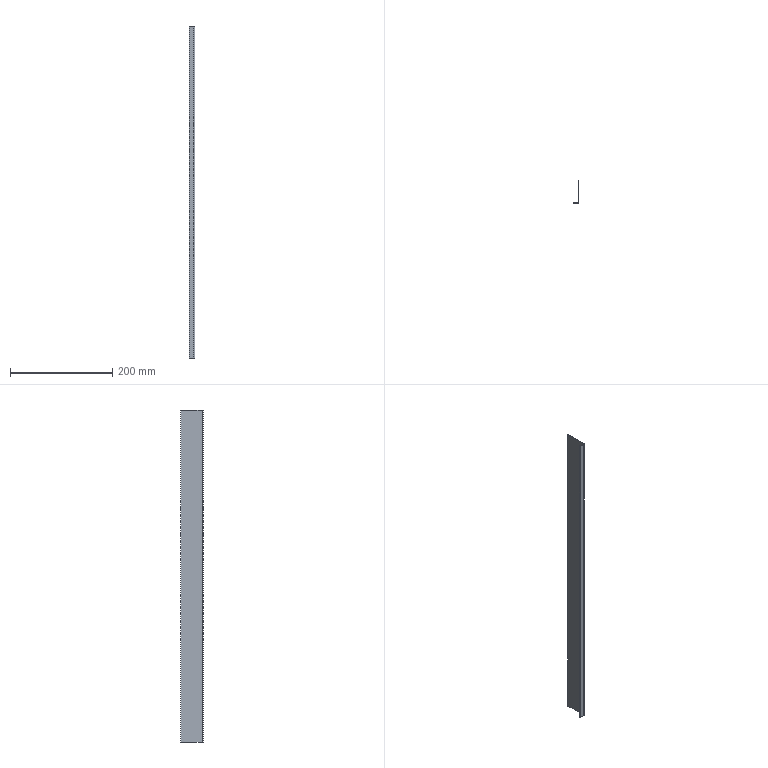Part | STEP file | 001-010-Waste drag chain mounting sheet metal | 1 solid | 14 faces | box 11.5 x 44.5 x 650 mm | volume 52405 mm3 | plane 12 | cylinder 2 | commonest cylinder face diameters 2 x1 5 x1
STEP:
#1=CARTESIAN_POINT('',(0.,0.,0.));
#2=DIRECTION('',(0.,0.,1.));
#3=DIRECTION('',(1.,0.,0.));
#4=AXIS2_PLACEMENT_3D('',#1,#2,#3);
#5=CARTESIAN_POINT('',(0.,1.,325.));
#6=VERTEX_POINT('',#5);
#7=CARTESIAN_POINT('',(1.5,1.,325.));
#8=VERTEX_POINT('',#7);
#9=CARTESIAN_POINT('',(0.,1.,325.));
#10=DIRECTION('',(1.,0.,0.));
#11=VECTOR('',#10,1.);
#12=LINE('',#9,#11);
#13=CARTESIAN_POINT('',(0.,1.,325.));
#14=DIRECTION('',(0.,0.,1.));
#15=DIRECTION('',(1.,0.,0.));
#16=AXIS2_PLACEMENT_3D('',#13,#14,#15);
#17=PLANE('',#16);
#18=CARTESIAN_POINT('',(0.,0.));
#19=DIRECTION('',(1.,0.));
#20=VECTOR('',#19,1.);
#21=LINE('',#18,#20);
#22=(GEOMETRIC_REPRESENTATION_CONTEXT(2)PARAMETRIC_REPRESENTATION_CONTEXT()REPRESENTATION_CONTEXT('',''));
#23=DEFINITIONAL_REPRESENTATION('',(#21),#22);
#24=PCURVE('',#17,#23);
#25=CARTESIAN_POINT('',(-1.,-1.5,325.));
#26=DIRECTION('',(0.,0.,1.));
#27=DIRECTION('',(1.,0.,0.));
#28=AXIS2_PLACEMENT_3D('',#25,#26,#27);
#29=PLANE('',#28);
#30=CARTESIAN_POINT('',(1.,2.5));
#31=DIRECTION('',(1.,0.));
#32=VECTOR('',#31,1.);
#33=LINE('',#30,#32);
#34=(GEOMETRIC_REPRESENTATION_CONTEXT(2)PARAMETRIC_REPRESENTATION_CONTEXT()REPRESENTATION_CONTEXT('',''));
#35=DEFINITIONAL_REPRESENTATION('',(#33),#34);
#36=PCURVE('',#29,#35);
#37=SURFACE_CURVE('',#12,(#24,#36),.PCURVE_S1.);
#38=EDGE_CURVE('',#6,#8,#37,.T.);
#39=ORIENTED_EDGE('',*,*,#38,.F.);
#40=CARTESIAN_POINT('',(-1.,0.,325.));
#41=VERTEX_POINT('',#40);
#42=CARTESIAN_POINT('',(-1.,1.,325.));
#43=DIRECTION('',(0.,0.,1.));
#44=DIRECTION('',(-1.,0.,0.));
#45=AXIS2_PLACEMENT_3D('',#42,#43,#44);
#46=CIRCLE('',#45,1.);
#47=CARTESIAN_POINT('',(-1.,0.));
#48=DIRECTION('',(-1.,0.));
#49=AXIS2_PLACEMENT_2D('',#47,#48);
#50=CIRCLE('',#49,1.);
#51=(GEOMETRIC_REPRESENTATION_CONTEXT(2)PARAMETRIC_REPRESENTATION_CONTEXT()REPRESENTATION_CONTEXT('',''));
#52=DEFINITIONAL_REPRESENTATION('',(#50),#51);
#53=PCURVE('',#17,#52);
#54=CARTESIAN_POINT('',(-1.,1.,325.));
#55=DIRECTION('',(0.,0.,-1.));
#56=DIRECTION('',(-1.,0.,0.));
#57=AXIS2_PLACEMENT_3D('',#54,#55,#56);
#58=CYLINDRICAL_SURFACE('',#57,1.);
#59=CARTESIAN_POINT('',(6.283,0.));
#60=DIRECTION('',(-1.,0.));
#61=VECTOR('',#60,1.);
#62=LINE('',#59,#61);
#63=(GEOMETRIC_REPRESENTATION_CONTEXT(2)PARAMETRIC_REPRESENTATION_CONTEXT()REPRESENTATION_CONTEXT('',''));
#64=DEFINITIONAL_REPRESENTATION('',(#62),#63);
#65=PCURVE('',#58,#64);
#66=SURFACE_CURVE('',#46,(#53,#65),.PCURVE_S1.);
#67=EDGE_CURVE('',#41,#6,#66,.T.);
#68=ORIENTED_EDGE('',*,*,#67,.F.);
#69=CARTESIAN_POINT('',(-1.,-1.5,325.));
#70=VERTEX_POINT('',#69);
#71=CARTESIAN_POINT('',(-1.,-1.5,325.));
#72=DIRECTION('',(0.,1.,0.));
#73=VECTOR('',#72,1.);
#74=LINE('',#71,#73);
#75=CARTESIAN_POINT('',(-1.,-2.5));
#76=DIRECTION('',(0.,1.));
#77=VECTOR('',#76,1.);
#78=LINE('',#75,#77);
#79=(GEOMETRIC_REPRESENTATION_CONTEXT(2)PARAMETRIC_REPRESENTATION_CONTEXT()REPRESENTATION_CONTEXT('',''));
#80=DEFINITIONAL_REPRESENTATION('',(#78),#79);
#81=PCURVE('',#17,#80);
#82=CARTESIAN_POINT('',(-1.,1.,325.));
#83=DIRECTION('',(0.,0.,-1.));
#84=DIRECTION('',(-1.,0.,0.));
#85=AXIS2_PLACEMENT_3D('',#82,#83,#84);
#86=PLANE('',#85);
#87=CARTESIAN_POINT('',(0.,-2.5));
#88=DIRECTION('',(0.,1.));
#89=VECTOR('',#88,1.);
#90=LINE('',#87,#89);
#91=(GEOMETRIC_REPRESENTATION_CONTEXT(2)PARAMETRIC_REPRESENTATION_CONTEXT()REPRESENTATION_CONTEXT('',''));
#92=DEFINITIONAL_REPRESENTATION('',(#90),#91);
#93=PCURVE('',#86,#92);
#94=SURFACE_CURVE('',#74,(#81,#93),.PCURVE_S1.);
#95=EDGE_CURVE('',#70,#41,#94,.T.);
#96=ORIENTED_EDGE('',*,*,#95,.F.);
#97=CARTESIAN_POINT('',(-1.,1.,325.));
#98=DIRECTION('',(0.,0.,1.));
#99=DIRECTION('',(1.,0.,0.));
#100=AXIS2_PLACEMENT_3D('',#97,#98,#99);
#101=CIRCLE('',#100,2.5);
#102=CARTESIAN_POINT('',(-1.,0.));
#103=DIRECTION('',(1.,0.));
#104=AXIS2_PLACEMENT_2D('',#102,#103);
#105=CIRCLE('',#104,2.5);
#106=(GEOMETRIC_REPRESENTATION_CONTEXT(2)PARAMETRIC_REPRESENTATION_CONTEXT()REPRESENTATION_CONTEXT('',''));
#107=DEFINITIONAL_REPRESENTATION('',(#105),#106);
#108=PCURVE('',#17,#107);
#109=CARTESIAN_POINT('',(-1.,1.,325.));
#110=DIRECTION('',(0.,0.,-1.));
#111=DIRECTION('',(-1.,0.,0.));
#112=AXIS2_PLACEMENT_3D('',#109,#110,#111);
#113=CYLINDRICAL_SURFACE('',#112,2.5);
#114=CARTESIAN_POINT('',(9.425,0.));
#115=DIRECTION('',(-1.,0.));
#116=VECTOR('',#115,1.);
#117=LINE('',#114,#116);
#118=(GEOMETRIC_REPRESENTATION_CONTEXT(2)PARAMETRIC_REPRESENTATION_CONTEXT()REPRESENTATION_CONTEXT('',''));
#119=DEFINITIONAL_REPRESENTATION('',(#117),#118);
#120=PCURVE('',#113,#119);
#121=SURFACE_CURVE('',#101,(#108,#120),.PCURVE_S1.);
#122=EDGE_CURVE('',#70,#8,#121,.T.);
#123=ORIENTED_EDGE('',*,*,#122,.T.);
#124=EDGE_LOOP('',(#39,#68,#96,#123));
#125=FACE_BOUND('',#124,.T.);
#126=ADVANCED_FACE('',(#125),#17,.T.);
#127=CARTESIAN_POINT('',(0.,43.,325.));
#128=VERTEX_POINT('',#127);
#129=CARTESIAN_POINT('',(0.,0.,325.));
#130=DIRECTION('',(0.,1.,0.));
#131=VECTOR('',#130,1.);
#132=LINE('',#129,#131);
#133=CARTESIAN_POINT('',(1.,1.5));
#134=DIRECTION('',(0.,1.));
#135=VECTOR('',#134,1.);
#136=LINE('',#133,#135);
#137=(GEOMETRIC_REPRESENTATION_CONTEXT(2)PARAMETRIC_REPRESENTATION_CONTEXT()REPRESENTATION_CONTEXT('',''));
#138=DEFINITIONAL_REPRESENTATION('',(#136),#137);
#139=PCURVE('',#29,#138);
#140=CARTESIAN_POINT('',(0.,0.,325.));
#141=DIRECTION('',(-1.,0.,0.));
#142=DIRECTION('',(0.,0.,1.));
#143=AXIS2_PLACEMENT_3D('',#140,#141,#142);
#144=PLANE('',#143);
#145=CARTESIAN_POINT('',(0.,0.));
#146=DIRECTION('',(0.,1.));
#147=VECTOR('',#146,1.);
#148=LINE('',#145,#147);
#149=(GEOMETRIC_REPRESENTATION_CONTEXT(2)PARAMETRIC_REPRESENTATION_CONTEXT()REPRESENTATION_CONTEXT('',''));
#150=DEFINITIONAL_REPRESENTATION('',(#148),#149);
#151=PCURVE('',#144,#150);
#152=SURFACE_CURVE('',#132,(#139,#151),.PCURVE_S1.);
#153=EDGE_CURVE('',#6,#128,#152,.T.);
#154=ORIENTED_EDGE('',*,*,#153,.F.);
#155=ORIENTED_EDGE('',*,*,#38,.T.);
#156=CARTESIAN_POINT('',(1.5,43.,325.));
#157=VERTEX_POINT('',#156);
#158=CARTESIAN_POINT('',(1.5,0.,325.));
#159=DIRECTION('',(0.,1.,0.));
#160=VECTOR('',#159,1.);
#161=LINE('',#158,#160);
#162=CARTESIAN_POINT('',(2.5,1.5));
#163=DIRECTION('',(0.,1.));
#164=VECTOR('',#163,1.);
#165=LINE('',#162,#164);
#166=(GEOMETRIC_REPRESENTATION_CONTEXT(2)PARAMETRIC_REPRESENTATION_CONTEXT()REPRESENTATION_CONTEXT('',''));
#167=DEFINITIONAL_REPRESENTATION('',(#165),#166);
#168=PCURVE('',#29,#167);
#169=CARTESIAN_POINT('',(1.5,0.,325.));
#170=DIRECTION('',(-1.,0.,0.));
#171=DIRECTION('',(0.,0.,1.));
#172=AXIS2_PLACEMENT_3D('',#169,#170,#171);
#173=PLANE('',#172);
#174=CARTESIAN_POINT('',(0.,0.));
#175=DIRECTION('',(0.,1.));
#176=VECTOR('',#175,1.);
#177=LINE('',#174,#176);
#178=(GEOMETRIC_REPRESENTATION_CONTEXT(2)PARAMETRIC_REPRESENTATION_CONTEXT()REPRESENTATION_CONTEXT('',''));
#179=DEFINITIONAL_REPRESENTATION('',(#177),#178);
#180=PCURVE('',#173,#179);
#181=SURFACE_CURVE('',#161,(#168,#180),.PCURVE_S1.);
#182=EDGE_CURVE('',#8,#157,#181,.T.);
#183=ORIENTED_EDGE('',*,*,#182,.T.);
#184=CARTESIAN_POINT('',(0.,43.,325.));
#185=DIRECTION('',(1.,0.,0.));
#186=VECTOR('',#185,1.);
#187=LINE('',#184,#186);
#188=CARTESIAN_POINT('',(1.,44.5));
#189=DIRECTION('',(1.,0.));
#190=VECTOR('',#189,1.);
#191=LINE('',#188,#190);
#192=(GEOMETRIC_REPRESENTATION_CONTEXT(2)PARAMETRIC_REPRESENTATION_CONTEXT()REPRESENTATION_CONTEXT('',''));
#193=DEFINITIONAL_REPRESENTATION('',(#191),#192);
#194=PCURVE('',#29,#193);
#195=CARTESIAN_POINT('',(0.,43.,325.));
#196=DIRECTION('',(0.,1.,0.));
#197=DIRECTION('',(0.,0.,1.));
#198=AXIS2_PLACEMENT_3D('',#195,#196,#197);
#199=PLANE('',#198);
#200=CARTESIAN_POINT('',(0.,0.));
#201=DIRECTION('',(0.,1.));
#202=VECTOR('',#201,1.);
#203=LINE('',#200,#202);
#204=(GEOMETRIC_REPRESENTATION_CONTEXT(2)PARAMETRIC_REPRESENTATION_CONTEXT()REPRESENTATION_CONTEXT('',''));
#205=DEFINITIONAL_REPRESENTATION('',(#203),#204);
#206=PCURVE('',#199,#205);
#207=SURFACE_CURVE('',#187,(#194,#206),.PCURVE_S1.);
#208=EDGE_CURVE('',#128,#157,#207,.T.);
#209=ORIENTED_EDGE('',*,*,#208,.F.);
#210=EDGE_LOOP('',(#154,#155,#183,#209));
#211=FACE_BOUND('',#210,.T.);
#212=ADVANCED_FACE('',(#211),#29,.T.);
#213=CARTESIAN_POINT('',(-1.,0.,-325.));
#214=VERTEX_POINT('',#213);
#215=CARTESIAN_POINT('',(-1.,-1.5,-325.));
#216=VERTEX_POINT('',#215);
#217=CARTESIAN_POINT('',(-1.,0.,-325.));
#218=DIRECTION('',(0.,-1.,0.));
#219=VECTOR('',#218,1.);
#220=LINE('',#217,#219);
#221=CARTESIAN_POINT('',(-1.,0.,-325.));
#222=DIRECTION('',(0.,0.,-1.));
#223=DIRECTION('',(-1.,0.,0.));
#224=AXIS2_PLACEMENT_3D('',#221,#222,#223);
#225=PLANE('',#224);
#226=CARTESIAN_POINT('',(0.,0.));
#227=DIRECTION('',(0.,-1.));
#228=VECTOR('',#227,1.);
#229=LINE('',#226,#228);
#230=(GEOMETRIC_REPRESENTATION_CONTEXT(2)PARAMETRIC_REPRESENTATION_CONTEXT()REPRESENTATION_CONTEXT('',''));
#231=DEFINITIONAL_REPRESENTATION('',(#229),#230);
#232=PCURVE('',#225,#231);
#233=CARTESIAN_POINT('',(1.5,1.,-325.));
#234=DIRECTION('',(0.,0.,-1.));
#235=DIRECTION('',(-1.,0.,0.));
#236=AXIS2_PLACEMENT_3D('',#233,#234,#235);
#237=PLANE('',#236);
#238=CARTESIAN_POINT('',(2.5,-1.));
#239=DIRECTION('',(0.,-1.));
#240=VECTOR('',#239,1.);
#241=LINE('',#238,#240);
#242=(GEOMETRIC_REPRESENTATION_CONTEXT(2)PARAMETRIC_REPRESENTATION_CONTEXT()REPRESENTATION_CONTEXT('',''));
#243=DEFINITIONAL_REPRESENTATION('',(#241),#242);
#244=PCURVE('',#237,#243);
#245=SURFACE_CURVE('',#220,(#232,#244),.PCURVE_S1.);
#246=EDGE_CURVE('',#214,#216,#245,.T.);
#247=ORIENTED_EDGE('',*,*,#246,.F.);
#248=CARTESIAN_POINT('',(0.,1.,-325.));
#249=VERTEX_POINT('',#248);
#250=CARTESIAN_POINT('',(-1.,1.,-325.));
#251=DIRECTION('',(0.,0.,1.));
#252=DIRECTION('',(-1.,0.,0.));
#253=AXIS2_PLACEMENT_3D('',#250,#251,#252);
#254=CIRCLE('',#253,1.);
#255=CARTESIAN_POINT('',(1.,1.));
#256=CARTESIAN_POINT('',(1.,-0.7321));
#257=CARTESIAN_POINT('',(-0.5,0.134));
#258=CARTESIAN_POINT('',(-2.,1.));
#259=CARTESIAN_POINT('',(-0.5,1.866));
#260=CARTESIAN_POINT('',(1.,2.732));
#261=CARTESIAN_POINT('',(1.,1.));
#262=(BOUNDED_CURVE()B_SPLINE_CURVE(2,(#255,#256,#257,#258,#259,#260,#261),.UNSPECIFIED.,.T.,.F.)B_SPLINE_CURVE_WITH_KNOTS((1,2,2,2,2,1),(-2.094,0.,2.094,4.189,6.283,8.378),.UNSPECIFIED.)CURVE()GEOMETRIC_REPRESENTATION_ITEM()RATIONAL_B_SPLINE_CURVE((1.,0.5,1.,0.5,1.,0.5,1.))REPRESENTATION_ITEM(''));
#263=(GEOMETRIC_REPRESENTATION_CONTEXT(2)PARAMETRIC_REPRESENTATION_CONTEXT()REPRESENTATION_CONTEXT('',''));
#264=DEFINITIONAL_REPRESENTATION('',(#262),#263);
#265=PCURVE('',#225,#264);
#266=CARTESIAN_POINT('',(6.283,650.));
#267=DIRECTION('',(-1.,0.));
#268=VECTOR('',#267,1.);
#269=LINE('',#266,#268);
#270=(GEOMETRIC_REPRESENTATION_CONTEXT(2)PARAMETRIC_REPRESENTATION_CONTEXT()REPRESENTATION_CONTEXT('',''));
#271=DEFINITIONAL_REPRESENTATION('',(#269),#270);
#272=PCURVE('',#58,#271);
#273=SURFACE_CURVE('',#254,(#265,#272),.PCURVE_S1.);
#274=EDGE_CURVE('',#214,#249,#273,.T.);
#275=ORIENTED_EDGE('',*,*,#274,.T.);
#276=CARTESIAN_POINT('',(1.5,1.,-325.));
#277=VERTEX_POINT('',#276);
#278=CARTESIAN_POINT('',(1.5,1.,-325.));
#279=DIRECTION('',(-1.,0.,0.));
#280=VECTOR('',#279,1.);
#281=LINE('',#278,#280);
#282=CARTESIAN_POINT('',(-2.5,1.));
#283=DIRECTION('',(1.,0.));
#284=VECTOR('',#283,1.);
#285=LINE('',#282,#284);
#286=(GEOMETRIC_REPRESENTATION_CONTEXT(2)PARAMETRIC_REPRESENTATION_CONTEXT()REPRESENTATION_CONTEXT('',''));
#287=DEFINITIONAL_REPRESENTATION('',(#285),#286);
#288=PCURVE('',#225,#287);
#289=CARTESIAN_POINT('',(-1.,1.,-325.));
#290=DIRECTION('',(0.,0.,-1.));
#291=DIRECTION('',(-1.,0.,0.));
#292=AXIS2_PLACEMENT_3D('',#289,#290,#291);
#293=PLANE('',#292);
#294=CARTESIAN_POINT('',(-2.5,0.));
#295=DIRECTION('',(1.,0.));
#296=VECTOR('',#295,1.);
#297=LINE('',#294,#296);
#298=(GEOMETRIC_REPRESENTATION_CONTEXT(2)PARAMETRIC_REPRESENTATION_CONTEXT()REPRESENTATION_CONTEXT('',''));
#299=DEFINITIONAL_REPRESENTATION('',(#297),#298);
#300=PCURVE('',#293,#299);
#301=SURFACE_CURVE('',#281,(#288,#300),.PCURVE_S1.);
#302=EDGE_CURVE('',#277,#249,#301,.T.);
#303=ORIENTED_EDGE('',*,*,#302,.F.);
#304=CARTESIAN_POINT('',(-1.,1.,-325.));
#305=DIRECTION('',(0.,0.,1.));
#306=DIRECTION('',(1.,0.,0.));
#307=AXIS2_PLACEMENT_3D('',#304,#305,#306);
#308=CIRCLE('',#307,2.5);
#309=CARTESIAN_POINT('',(-2.5,1.));
#310=CARTESIAN_POINT('',(-2.5,5.33));
#311=CARTESIAN_POINT('',(1.25,3.165));
#312=CARTESIAN_POINT('',(5.,1.));
#313=CARTESIAN_POINT('',(1.25,-1.165));
#314=CARTESIAN_POINT('',(-2.5,-3.33));
#315=CARTESIAN_POINT('',(-2.5,1.));
#316=(BOUNDED_CURVE()B_SPLINE_CURVE(2,(#309,#310,#311,#312,#313,#314,#315),.UNSPECIFIED.,.T.,.F.)B_SPLINE_CURVE_WITH_KNOTS((1,2,2,2,2,1),(-2.094,0.,2.094,4.189,6.283,8.378),.UNSPECIFIED.)CURVE()GEOMETRIC_REPRESENTATION_ITEM()RATIONAL_B_SPLINE_CURVE((1.,0.5,1.,0.5,1.,0.5,1.))REPRESENTATION_ITEM(''));
#317=(GEOMETRIC_REPRESENTATION_CONTEXT(2)PARAMETRIC_REPRESENTATION_CONTEXT()REPRESENTATION_CONTEXT('',''));
#318=DEFINITIONAL_REPRESENTATION('',(#316),#317);
#319=PCURVE('',#225,#318);
#320=CARTESIAN_POINT('',(9.425,650.));
#321=DIRECTION('',(-1.,0.));
#322=VECTOR('',#321,1.);
#323=LINE('',#320,#322);
#324=(GEOMETRIC_REPRESENTATION_CONTEXT(2)PARAMETRIC_REPRESENTATION_CONTEXT()REPRESENTATION_CONTEXT('',''));
#325=DEFINITIONAL_REPRESENTATION('',(#323),#324);
#326=PCURVE('',#113,#325);
#327=SURFACE_CURVE('',#308,(#319,#326),.PCURVE_S1.);
#328=EDGE_CURVE('',#216,#277,#327,.T.);
#329=ORIENTED_EDGE('',*,*,#328,.F.);
#330=EDGE_LOOP('',(#247,#275,#303,#329));
#331=FACE_BOUND('',#330,.T.);
#332=ADVANCED_FACE('',(#331),#225,.T.);
#333=CARTESIAN_POINT('',(-10.,0.,-325.));
#334=VERTEX_POINT('',#333);
#335=CARTESIAN_POINT('',(0.,0.,-325.));
#336=DIRECTION('',(1.,0.,0.));
#337=VECTOR('',#336,1.);
#338=LINE('',#335,#337);
#339=CARTESIAN_POINT('',(1.5,-1.));
#340=DIRECTION('',(-1.,0.));
#341=VECTOR('',#340,1.);
#342=LINE('',#339,#341);
#343=(GEOMETRIC_REPRESENTATION_CONTEXT(2)PARAMETRIC_REPRESENTATION_CONTEXT()REPRESENTATION_CONTEXT('',''));
#344=DEFINITIONAL_REPRESENTATION('',(#342),#343);
#345=PCURVE('',#237,#344);
#346=CARTESIAN_POINT('',(0.,0.,325.));
#347=DIRECTION('',(0.,1.,0.));
#348=DIRECTION('',(0.,0.,1.));
#349=AXIS2_PLACEMENT_3D('',#346,#347,#348);
#350=PLANE('',#349);
#351=CARTESIAN_POINT('',(-650.,0.));
#352=DIRECTION('',(0.,1.));
#353=VECTOR('',#352,1.);
#354=LINE('',#351,#353);
#355=(GEOMETRIC_REPRESENTATION_CONTEXT(2)PARAMETRIC_REPRESENTATION_CONTEXT()REPRESENTATION_CONTEXT('',''));
#356=DEFINITIONAL_REPRESENTATION('',(#354),#355);
#357=PCURVE('',#350,#356);
#358=SURFACE_CURVE('',#338,(#345,#357),.PCURVE_S1.);
#359=EDGE_CURVE('',#334,#214,#358,.T.);
#360=ORIENTED_EDGE('',*,*,#359,.T.);
#361=ORIENTED_EDGE('',*,*,#246,.T.);
#362=CARTESIAN_POINT('',(-10.,-1.5,-325.));
#363=VERTEX_POINT('',#362);
#364=CARTESIAN_POINT('',(0.,-1.5,-325.));
#365=DIRECTION('',(1.,0.,0.));
#366=VECTOR('',#365,1.);
#367=LINE('',#364,#366);
#368=CARTESIAN_POINT('',(1.5,-2.5));
#369=DIRECTION('',(-1.,0.));
#370=VECTOR('',#369,1.);
#371=LINE('',#368,#370);
#372=(GEOMETRIC_REPRESENTATION_CONTEXT(2)PARAMETRIC_REPRESENTATION_CONTEXT()REPRESENTATION_CONTEXT('',''));
#373=DEFINITIONAL_REPRESENTATION('',(#371),#372);
#374=PCURVE('',#237,#373);
#375=CARTESIAN_POINT('',(0.,-1.5,325.));
#376=DIRECTION('',(0.,1.,0.));
#377=DIRECTION('',(0.,0.,1.));
#378=AXIS2_PLACEMENT_3D('',#375,#376,#377);
#379=PLANE('',#378);
#380=CARTESIAN_POINT('',(-650.,0.));
#381=DIRECTION('',(0.,1.));
#382=VECTOR('',#381,1.);
#383=LINE('',#380,#382);
#384=(GEOMETRIC_REPRESENTATION_CONTEXT(2)PARAMETRIC_REPRESENTATION_CONTEXT()REPRESENTATION_CONTEXT('',''));
#385=DEFINITIONAL_REPRESENTATION('',(#383),#384);
#386=PCURVE('',#379,#385);
#387=SURFACE_CURVE('',#367,(#374,#386),.PCURVE_S1.);
#388=EDGE_CURVE('',#363,#216,#387,.T.);
#389=ORIENTED_EDGE('',*,*,#388,.F.);
#390=CARTESIAN_POINT('',(-10.,-1.5,-325.));
#391=DIRECTION('',(0.,1.,0.));
#392=VECTOR('',#391,1.);
#393=LINE('',#390,#392);
#394=CARTESIAN_POINT('',(11.5,-2.5));
#395=DIRECTION('',(0.,1.));
#396=VECTOR('',#395,1.);
#397=LINE('',#394,#396);
#398=(GEOMETRIC_REPRESENTATION_CONTEXT(2)PARAMETRIC_REPRESENTATION_CONTEXT()REPRESENTATION_CONTEXT('',''));
#399=DEFINITIONAL_REPRESENTATION('',(#397),#398);
#400=PCURVE('',#237,#399);
#401=CARTESIAN_POINT('',(-10.,-1.5,325.));
#402=DIRECTION('',(-1.,0.,0.));
#403=DIRECTION('',(0.,0.,1.));
#404=AXIS2_PLACEMENT_3D('',#401,#402,#403);
#405=PLANE('',#404);
#406=CARTESIAN_POINT('',(-650.,0.));
#407=DIRECTION('',(0.,1.));
#408=VECTOR('',#407,1.);
#409=LINE('',#406,#408);
#410=(GEOMETRIC_REPRESENTATION_CONTEXT(2)PARAMETRIC_REPRESENTATION_CONTEXT()REPRESENTATION_CONTEXT('',''));
#411=DEFINITIONAL_REPRESENTATION('',(#409),#410);
#412=PCURVE('',#405,#411);
#413=SURFACE_CURVE('',#393,(#400,#412),.PCURVE_S1.);
#414=EDGE_CURVE('',#363,#334,#413,.T.);
#415=ORIENTED_EDGE('',*,*,#414,.T.);
#416=EDGE_LOOP('',(#360,#361,#389,#415));
#417=FACE_BOUND('',#416,.T.);
#418=ADVANCED_FACE('',(#417),#237,.T.);
#419=CARTESIAN_POINT('',(1.5,43.,-325.));
#420=VERTEX_POINT('',#419);
#421=CARTESIAN_POINT('',(1.5,0.,-325.));
#422=DIRECTION('',(0.,1.,0.));
#423=VECTOR('',#422,1.);
#424=LINE('',#421,#423);
#425=CARTESIAN_POINT('',(-650.,0.));
#426=DIRECTION('',(0.,1.));
#427=VECTOR('',#426,1.);
#428=LINE('',#425,#427);
#429=(GEOMETRIC_REPRESENTATION_CONTEXT(2)PARAMETRIC_REPRESENTATION_CONTEXT()REPRESENTATION_CONTEXT('',''));
#430=DEFINITIONAL_REPRESENTATION('',(#428),#429);
#431=PCURVE('',#173,#430);
#432=CARTESIAN_POINT('',(-2.5,-1.));
#433=DIRECTION('',(0.,1.));
#434=VECTOR('',#433,1.);
#435=LINE('',#432,#434);
#436=(GEOMETRIC_REPRESENTATION_CONTEXT(2)PARAMETRIC_REPRESENTATION_CONTEXT()REPRESENTATION_CONTEXT('',''));
#437=DEFINITIONAL_REPRESENTATION('',(#435),#436);
#438=PCURVE('',#293,#437);
#439=SURFACE_CURVE('',#424,(#431,#438),.PCURVE_S1.);
#440=EDGE_CURVE('',#277,#420,#439,.T.);
#441=ORIENTED_EDGE('',*,*,#440,.T.);
#442=CARTESIAN_POINT('',(1.5,43.,325.));
#443=DIRECTION('',(0.,0.,-1.));
#444=VECTOR('',#443,1.);
#445=LINE('',#442,#444);
#446=CARTESIAN_POINT('',(0.,43.));
#447=DIRECTION('',(-1.,0.));
#448=VECTOR('',#447,1.);
#449=LINE('',#446,#448);
#450=(GEOMETRIC_REPRESENTATION_CONTEXT(2)PARAMETRIC_REPRESENTATION_CONTEXT()REPRESENTATION_CONTEXT('',''));
#451=DEFINITIONAL_REPRESENTATION('',(#449),#450);
#452=PCURVE('',#173,#451);
#453=CARTESIAN_POINT('',(0.,1.5));
#454=DIRECTION('',(-1.,0.));
#455=VECTOR('',#454,1.);
#456=LINE('',#453,#455);
#457=(GEOMETRIC_REPRESENTATION_CONTEXT(2)PARAMETRIC_REPRESENTATION_CONTEXT()REPRESENTATION_CONTEXT('',''));
#458=DEFINITIONAL_REPRESENTATION('',(#456),#457);
#459=PCURVE('',#199,#458);
#460=SURFACE_CURVE('',#445,(#452,#459),.PCURVE_S1.);
#461=EDGE_CURVE('',#157,#420,#460,.T.);
#462=ORIENTED_EDGE('',*,*,#461,.F.);
#463=ORIENTED_EDGE('',*,*,#182,.F.);
#464=CARTESIAN_POINT('',(1.5,1.,325.));
#465=DIRECTION('',(0.,0.,-1.));
#466=VECTOR('',#465,1.);
#467=LINE('',#464,#466);
#468=CARTESIAN_POINT('',(0.,1.));
#469=DIRECTION('',(-1.,0.));
#470=VECTOR('',#469,1.);
#471=LINE('',#468,#470);
#472=(GEOMETRIC_REPRESENTATION_CONTEXT(2)PARAMETRIC_REPRESENTATION_CONTEXT()REPRESENTATION_CONTEXT('',''));
#473=DEFINITIONAL_REPRESENTATION('',(#471),#472);
#474=PCURVE('',#173,#473);
#475=CARTESIAN_POINT('',(3.142,0.));
#476=DIRECTION('',(0.,1.));
#477=VECTOR('',#476,1.);
#478=LINE('',#475,#477);
#479=(GEOMETRIC_REPRESENTATION_CONTEXT(2)PARAMETRIC_REPRESENTATION_CONTEXT()REPRESENTATION_CONTEXT('',''));
#480=DEFINITIONAL_REPRESENTATION('',(#478),#479);
#481=PCURVE('',#113,#480);
#482=SURFACE_CURVE('',#467,(#474,#481),.PCURVE_S1.);
#483=EDGE_CURVE('',#8,#277,#482,.T.);
#484=ORIENTED_EDGE('',*,*,#483,.T.);
#485=EDGE_LOOP('',(#441,#462,#463,#484));
#486=FACE_BOUND('',#485,.T.);
#487=ADVANCED_FACE('',(#486),#173,.F.);
#488=CARTESIAN_POINT('',(0.,43.,-325.));
#489=VERTEX_POINT('',#488);
#490=CARTESIAN_POINT('',(0.,43.,-325.));
#491=DIRECTION('',(1.,0.,0.));
#492=VECTOR('',#491,1.);
#493=LINE('',#490,#492);
#494=CARTESIAN_POINT('',(-650.,0.));
#495=DIRECTION('',(0.,1.));
#496=VECTOR('',#495,1.);
#497=LINE('',#494,#496);
#498=(GEOMETRIC_REPRESENTATION_CONTEXT(2)PARAMETRIC_REPRESENTATION_CONTEXT()REPRESENTATION_CONTEXT('',''));
#499=DEFINITIONAL_REPRESENTATION('',(#497),#498);
#500=PCURVE('',#199,#499);
#501=CARTESIAN_POINT('',(-1.,42.));
#502=DIRECTION('',(-1.,0.));
#503=VECTOR('',#502,1.);
#504=LINE('',#501,#503);
#505=(GEOMETRIC_REPRESENTATION_CONTEXT(2)PARAMETRIC_REPRESENTATION_CONTEXT()REPRESENTATION_CONTEXT('',''));
#506=DEFINITIONAL_REPRESENTATION('',(#504),#505);
#507=PCURVE('',#293,#506);
#508=SURFACE_CURVE('',#493,(#500,#507),.PCURVE_S1.);
#509=EDGE_CURVE('',#489,#420,#508,.T.);
#510=ORIENTED_EDGE('',*,*,#509,.F.);
#511=CARTESIAN_POINT('',(0.,43.,325.));
#512=DIRECTION('',(0.,0.,-1.));
#513=VECTOR('',#512,1.);
#514=LINE('',#511,#513);
#515=CARTESIAN_POINT('',(0.,0.));
#516=DIRECTION('',(-1.,0.));
#517=VECTOR('',#516,1.);
#518=LINE('',#515,#517);
#519=(GEOMETRIC_REPRESENTATION_CONTEXT(2)PARAMETRIC_REPRESENTATION_CONTEXT()REPRESENTATION_CONTEXT('',''));
#520=DEFINITIONAL_REPRESENTATION('',(#518),#519);
#521=PCURVE('',#199,#520);
#522=CARTESIAN_POINT('',(0.,43.));
#523=DIRECTION('',(-1.,0.));
#524=VECTOR('',#523,1.);
#525=LINE('',#522,#524);
#526=(GEOMETRIC_REPRESENTATION_CONTEXT(2)PARAMETRIC_REPRESENTATION_CONTEXT()REPRESENTATION_CONTEXT('',''));
#527=DEFINITIONAL_REPRESENTATION('',(#525),#526);
#528=PCURVE('',#144,#527);
#529=SURFACE_CURVE('',#514,(#521,#528),.PCURVE_S1.);
#530=EDGE_CURVE('',#128,#489,#529,.T.);
#531=ORIENTED_EDGE('',*,*,#530,.F.);
#532=ORIENTED_EDGE('',*,*,#208,.T.);
#533=ORIENTED_EDGE('',*,*,#461,.T.);
#534=EDGE_LOOP('',(#510,#531,#532,#533));
#535=FACE_BOUND('',#534,.T.);
#536=ADVANCED_FACE('',(#535),#199,.T.);
#537=CARTESIAN_POINT('',(0.,0.,-325.));
#538=DIRECTION('',(0.,1.,0.));
#539=VECTOR('',#538,1.);
#540=LINE('',#537,#539);
#541=CARTESIAN_POINT('',(-650.,0.));
#542=DIRECTION('',(0.,1.));
#543=VECTOR('',#542,1.);
#544=LINE('',#541,#543);
#545=(GEOMETRIC_REPRESENTATION_CONTEXT(2)PARAMETRIC_REPRESENTATION_CONTEXT()REPRESENTATION_CONTEXT('',''));
#546=DEFINITIONAL_REPRESENTATION('',(#544),#545);
#547=PCURVE('',#144,#546);
#548=CARTESIAN_POINT('',(-1.,-1.));
#549=DIRECTION('',(0.,1.));
#550=VECTOR('',#549,1.);
#551=LINE('',#548,#550);
#552=(GEOMETRIC_REPRESENTATION_CONTEXT(2)PARAMETRIC_REPRESENTATION_CONTEXT()REPRESENTATION_CONTEXT('',''));
#553=DEFINITIONAL_REPRESENTATION('',(#551),#552);
#554=PCURVE('',#293,#553);
#555=SURFACE_CURVE('',#540,(#547,#554),.PCURVE_S1.);
#556=EDGE_CURVE('',#249,#489,#555,.T.);
#557=ORIENTED_EDGE('',*,*,#556,.F.);
#558=CARTESIAN_POINT('',(0.,1.,325.));
#559=DIRECTION('',(0.,0.,-1.));
#560=VECTOR('',#559,1.);
#561=LINE('',#558,#560);
#562=CARTESIAN_POINT('',(0.,1.));
#563=DIRECTION('',(-1.,0.));
#564=VECTOR('',#563,1.);
#565=LINE('',#562,#564);
#566=(GEOMETRIC_REPRESENTATION_CONTEXT(2)PARAMETRIC_REPRESENTATION_CONTEXT()REPRESENTATION_CONTEXT('',''));
#567=DEFINITIONAL_REPRESENTATION('',(#565),#566);
#568=PCURVE('',#144,#567);
#569=CARTESIAN_POINT('',(3.142,0.));
#570=DIRECTION('',(0.,1.));
#571=VECTOR('',#570,1.);
#572=LINE('',#569,#571);
#573=(GEOMETRIC_REPRESENTATION_CONTEXT(2)PARAMETRIC_REPRESENTATION_CONTEXT()REPRESENTATION_CONTEXT('',''));
#574=DEFINITIONAL_REPRESENTATION('',(#572),#573);
#575=PCURVE('',#58,#574);
#576=SURFACE_CURVE('',#561,(#568,#575),.PCURVE_S1.);
#577=EDGE_CURVE('',#6,#249,#576,.T.);
#578=ORIENTED_EDGE('',*,*,#577,.F.);
#579=ORIENTED_EDGE('',*,*,#153,.T.);
#580=ORIENTED_EDGE('',*,*,#530,.T.);
#581=EDGE_LOOP('',(#557,#578,#579,#580));
#582=FACE_BOUND('',#581,.T.);
#583=ADVANCED_FACE('',(#582),#144,.T.);
#584=ORIENTED_EDGE('',*,*,#577,.F.);
#585=ORIENTED_EDGE('',*,*,#67,.F.);
#586=CARTESIAN_POINT('',(-1.,0.,325.));
#587=DIRECTION('',(0.,0.,-1.));
#588=VECTOR('',#587,1.);
#589=LINE('',#586,#588);
#590=CARTESIAN_POINT('',(4.712,0.));
#591=DIRECTION('',(0.,1.));
#592=VECTOR('',#591,1.);
#593=LINE('',#590,#592);
#594=(GEOMETRIC_REPRESENTATION_CONTEXT(2)PARAMETRIC_REPRESENTATION_CONTEXT()REPRESENTATION_CONTEXT('',''));
#595=DEFINITIONAL_REPRESENTATION('',(#593),#594);
#596=PCURVE('',#58,#595);
#597=CARTESIAN_POINT('',(0.,-1.));
#598=DIRECTION('',(-1.,0.));
#599=VECTOR('',#598,1.);
#600=LINE('',#597,#599);
#601=(GEOMETRIC_REPRESENTATION_CONTEXT(2)PARAMETRIC_REPRESENTATION_CONTEXT()REPRESENTATION_CONTEXT('',''));
#602=DEFINITIONAL_REPRESENTATION('',(#600),#601);
#603=PCURVE('',#350,#602);
#604=SURFACE_CURVE('',#589,(#596,#603),.PCURVE_S1.);
#605=EDGE_CURVE('',#41,#214,#604,.T.);
#606=ORIENTED_EDGE('',*,*,#605,.T.);
#607=ORIENTED_EDGE('',*,*,#274,.T.);
#608=EDGE_LOOP('',(#584,#585,#606,#607));
#609=FACE_BOUND('',#608,.F.);
#610=ADVANCED_FACE('',(#609),#58,.F.);
#611=ORIENTED_EDGE('',*,*,#359,.F.);
#612=CARTESIAN_POINT('',(-10.,0.,325.));
#613=VERTEX_POINT('',#612);
#614=CARTESIAN_POINT('',(-10.,0.,325.));
#615=DIRECTION('',(0.,0.,-1.));
#616=VECTOR('',#615,1.);
#617=LINE('',#614,#616);
#618=CARTESIAN_POINT('',(0.,-10.));
#619=DIRECTION('',(-1.,0.));
#620=VECTOR('',#619,1.);
#621=LINE('',#618,#620);
#622=(GEOMETRIC_REPRESENTATION_CONTEXT(2)PARAMETRIC_REPRESENTATION_CONTEXT()REPRESENTATION_CONTEXT('',''));
#623=DEFINITIONAL_REPRESENTATION('',(#621),#622);
#624=PCURVE('',#350,#623);
#625=CARTESIAN_POINT('',(0.,1.5));
#626=DIRECTION('',(-1.,0.));
#627=VECTOR('',#626,1.);
#628=LINE('',#625,#627);
#629=(GEOMETRIC_REPRESENTATION_CONTEXT(2)PARAMETRIC_REPRESENTATION_CONTEXT()REPRESENTATION_CONTEXT('',''));
#630=DEFINITIONAL_REPRESENTATION('',(#628),#629);
#631=PCURVE('',#405,#630);
#632=SURFACE_CURVE('',#617,(#624,#631),.PCURVE_S1.);
#633=EDGE_CURVE('',#613,#334,#632,.T.);
#634=ORIENTED_EDGE('',*,*,#633,.F.);
#635=CARTESIAN_POINT('',(0.,0.,325.));
#636=DIRECTION('',(1.,0.,0.));
#637=VECTOR('',#636,1.);
#638=LINE('',#635,#637);
#639=CARTESIAN_POINT('',(0.,0.));
#640=DIRECTION('',(0.,1.));
#641=VECTOR('',#640,1.);
#642=LINE('',#639,#641);
#643=(GEOMETRIC_REPRESENTATION_CONTEXT(2)PARAMETRIC_REPRESENTATION_CONTEXT()REPRESENTATION_CONTEXT('',''));
#644=DEFINITIONAL_REPRESENTATION('',(#642),#643);
#645=PCURVE('',#350,#644);
#646=CARTESIAN_POINT('',(-1.,-1.));
#647=DIRECTION('',(-1.,0.));
#648=VECTOR('',#647,1.);
#649=LINE('',#646,#648);
#650=(GEOMETRIC_REPRESENTATION_CONTEXT(2)PARAMETRIC_REPRESENTATION_CONTEXT()REPRESENTATION_CONTEXT('',''));
#651=DEFINITIONAL_REPRESENTATION('',(#649),#650);
#652=PCURVE('',#86,#651);
#653=SURFACE_CURVE('',#638,(#645,#652),.PCURVE_S1.);
#654=EDGE_CURVE('',#613,#41,#653,.T.);
#655=ORIENTED_EDGE('',*,*,#654,.T.);
#656=ORIENTED_EDGE('',*,*,#605,.T.);
#657=EDGE_LOOP('',(#611,#634,#655,#656));
#658=FACE_BOUND('',#657,.T.);
#659=ADVANCED_FACE('',(#658),#350,.T.);
#660=ORIENTED_EDGE('',*,*,#414,.F.);
#661=CARTESIAN_POINT('',(-10.,-1.5,325.));
#662=VERTEX_POINT('',#661);
#663=CARTESIAN_POINT('',(-10.,-1.5,325.));
#664=DIRECTION('',(0.,0.,-1.));
#665=VECTOR('',#664,1.);
#666=LINE('',#663,#665);
#667=CARTESIAN_POINT('',(0.,0.));
#668=DIRECTION('',(-1.,0.));
#669=VECTOR('',#668,1.);
#670=LINE('',#667,#669);
#671=(GEOMETRIC_REPRESENTATION_CONTEXT(2)PARAMETRIC_REPRESENTATION_CONTEXT()REPRESENTATION_CONTEXT('',''));
#672=DEFINITIONAL_REPRESENTATION('',(#670),#671);
#673=PCURVE('',#405,#672);
#674=CARTESIAN_POINT('',(0.,-10.));
#675=DIRECTION('',(-1.,0.));
#676=VECTOR('',#675,1.);
#677=LINE('',#674,#676);
#678=(GEOMETRIC_REPRESENTATION_CONTEXT(2)PARAMETRIC_REPRESENTATION_CONTEXT()REPRESENTATION_CONTEXT('',''));
#679=DEFINITIONAL_REPRESENTATION('',(#677),#678);
#680=PCURVE('',#379,#679);
#681=SURFACE_CURVE('',#666,(#673,#680),.PCURVE_S1.);
#682=EDGE_CURVE('',#662,#363,#681,.T.);
#683=ORIENTED_EDGE('',*,*,#682,.F.);
#684=CARTESIAN_POINT('',(-10.,-1.5,325.));
#685=DIRECTION('',(0.,1.,0.));
#686=VECTOR('',#685,1.);
#687=LINE('',#684,#686);
#688=CARTESIAN_POINT('',(0.,0.));
#689=DIRECTION('',(0.,1.));
#690=VECTOR('',#689,1.);
#691=LINE('',#688,#690);
#692=(GEOMETRIC_REPRESENTATION_CONTEXT(2)PARAMETRIC_REPRESENTATION_CONTEXT()REPRESENTATION_CONTEXT('',''));
#693=DEFINITIONAL_REPRESENTATION('',(#691),#692);
#694=PCURVE('',#405,#693);
#695=CARTESIAN_POINT('',(9.,-2.5));
#696=DIRECTION('',(0.,1.));
#697=VECTOR('',#696,1.);
#698=LINE('',#695,#697);
#699=(GEOMETRIC_REPRESENTATION_CONTEXT(2)PARAMETRIC_REPRESENTATION_CONTEXT()REPRESENTATION_CONTEXT('',''));
#700=DEFINITIONAL_REPRESENTATION('',(#698),#699);
#701=PCURVE('',#86,#700);
#702=SURFACE_CURVE('',#687,(#694,#701),.PCURVE_S1.);
#703=EDGE_CURVE('',#662,#613,#702,.T.);
#704=ORIENTED_EDGE('',*,*,#703,.T.);
#705=ORIENTED_EDGE('',*,*,#633,.T.);
#706=EDGE_LOOP('',(#660,#683,#704,#705));
#707=FACE_BOUND('',#706,.T.);
#708=ADVANCED_FACE('',(#707),#405,.T.);
#709=ORIENTED_EDGE('',*,*,#388,.T.);
#710=CARTESIAN_POINT('',(-1.,-1.5,325.));
#711=DIRECTION('',(0.,0.,-1.));
#712=VECTOR('',#711,1.);
#713=LINE('',#710,#712);
#714=CARTESIAN_POINT('',(0.,-1.));
#715=DIRECTION('',(-1.,0.));
#716=VECTOR('',#715,1.);
#717=LINE('',#714,#716);
#718=(GEOMETRIC_REPRESENTATION_CONTEXT(2)PARAMETRIC_REPRESENTATION_CONTEXT()REPRESENTATION_CONTEXT('',''));
#719=DEFINITIONAL_REPRESENTATION('',(#717),#718);
#720=PCURVE('',#379,#719);
#721=CARTESIAN_POINT('',(4.712,0.));
#722=DIRECTION('',(0.,1.));
#723=VECTOR('',#722,1.);
#724=LINE('',#721,#723);
#725=(GEOMETRIC_REPRESENTATION_CONTEXT(2)PARAMETRIC_REPRESENTATION_CONTEXT()REPRESENTATION_CONTEXT('',''));
#726=DEFINITIONAL_REPRESENTATION('',(#724),#725);
#727=PCURVE('',#113,#726);
#728=SURFACE_CURVE('',#713,(#720,#727),.PCURVE_S1.);
#729=EDGE_CURVE('',#70,#216,#728,.T.);
#730=ORIENTED_EDGE('',*,*,#729,.F.);
#731=CARTESIAN_POINT('',(0.,-1.5,325.));
#732=DIRECTION('',(1.,0.,0.));
#733=VECTOR('',#732,1.);
#734=LINE('',#731,#733);
#735=CARTESIAN_POINT('',(0.,0.));
#736=DIRECTION('',(0.,1.));
#737=VECTOR('',#736,1.);
#738=LINE('',#735,#737);
#739=(GEOMETRIC_REPRESENTATION_CONTEXT(2)PARAMETRIC_REPRESENTATION_CONTEXT()REPRESENTATION_CONTEXT('',''));
#740=DEFINITIONAL_REPRESENTATION('',(#738),#739);
#741=PCURVE('',#379,#740);
#742=CARTESIAN_POINT('',(-1.,-2.5));
#743=DIRECTION('',(-1.,0.));
#744=VECTOR('',#743,1.);
#745=LINE('',#742,#744);
#746=(GEOMETRIC_REPRESENTATION_CONTEXT(2)PARAMETRIC_REPRESENTATION_CONTEXT()REPRESENTATION_CONTEXT('',''));
#747=DEFINITIONAL_REPRESENTATION('',(#745),#746);
#748=PCURVE('',#86,#747);
#749=SURFACE_CURVE('',#734,(#741,#748),.PCURVE_S1.);
#750=EDGE_CURVE('',#662,#70,#749,.T.);
#751=ORIENTED_EDGE('',*,*,#750,.F.);
#752=ORIENTED_EDGE('',*,*,#682,.T.);
#753=EDGE_LOOP('',(#709,#730,#751,#752));
#754=FACE_BOUND('',#753,.T.);
#755=ADVANCED_FACE('',(#754),#379,.F.);
#756=ORIENTED_EDGE('',*,*,#328,.T.);
#757=ORIENTED_EDGE('',*,*,#483,.F.);
#758=ORIENTED_EDGE('',*,*,#122,.F.);
#759=ORIENTED_EDGE('',*,*,#729,.T.);
#760=EDGE_LOOP('',(#756,#757,#758,#759));
#761=FACE_BOUND('',#760,.T.);
#762=ADVANCED_FACE('',(#761),#113,.T.);
#763=ORIENTED_EDGE('',*,*,#750,.T.);
#764=ORIENTED_EDGE('',*,*,#95,.T.);
#765=ORIENTED_EDGE('',*,*,#654,.F.);
#766=ORIENTED_EDGE('',*,*,#703,.F.);
#767=EDGE_LOOP('',(#763,#764,#765,#766));
#768=FACE_BOUND('',#767,.T.);
#769=ADVANCED_FACE('',(#768),#86,.F.);
#770=ORIENTED_EDGE('',*,*,#440,.F.);
#771=ORIENTED_EDGE('',*,*,#302,.T.);
#772=ORIENTED_EDGE('',*,*,#556,.T.);
#773=ORIENTED_EDGE('',*,*,#509,.T.);
#774=EDGE_LOOP('',(#770,#771,#772,#773));
#775=FACE_BOUND('',#774,.T.);
#776=ADVANCED_FACE('',(#775),#293,.T.);
#777=CLOSED_SHELL('',(#126,#212,#332,#418,#487,#536,#583,#610,#659,#708,#755,#762,#769,#776));
#778=MANIFOLD_SOLID_BREP('',#777);
#779=(LENGTH_UNIT()NAMED_UNIT(*)SI_UNIT(.MILLI.,.METRE.));
#780=UNCERTAINTY_MEASURE_WITH_UNIT(LENGTH_MEASURE(0.0000001),#779,'','');
#781=(NAMED_UNIT(*)PLANE_ANGLE_UNIT()SI_UNIT($,.RADIAN.));
#782=(NAMED_UNIT(*)SI_UNIT($,.STERADIAN.)SOLID_ANGLE_UNIT());
#783=(GEOMETRIC_REPRESENTATION_CONTEXT(3)GLOBAL_UNCERTAINTY_ASSIGNED_CONTEXT((#780))GLOBAL_UNIT_ASSIGNED_CONTEXT((#779,#781,#782))REPRESENTATION_CONTEXT('',''));
#784=ADVANCED_BREP_SHAPE_REPRESENTATION('',(#4,#778),#783);